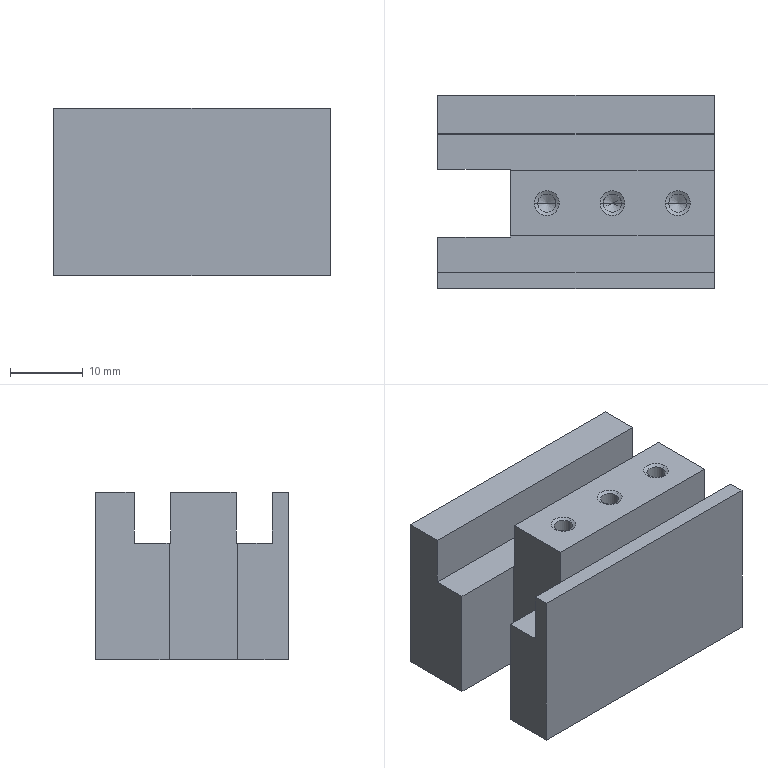Part | NX | 1 solid | 54 faces | box 38 x 26.5 x 23 mm | volume 17903 mm3 | cone 24 | plane 18 | cylinder 12 | commonest cylinder face diameters 2.5 x6 3.3 x6